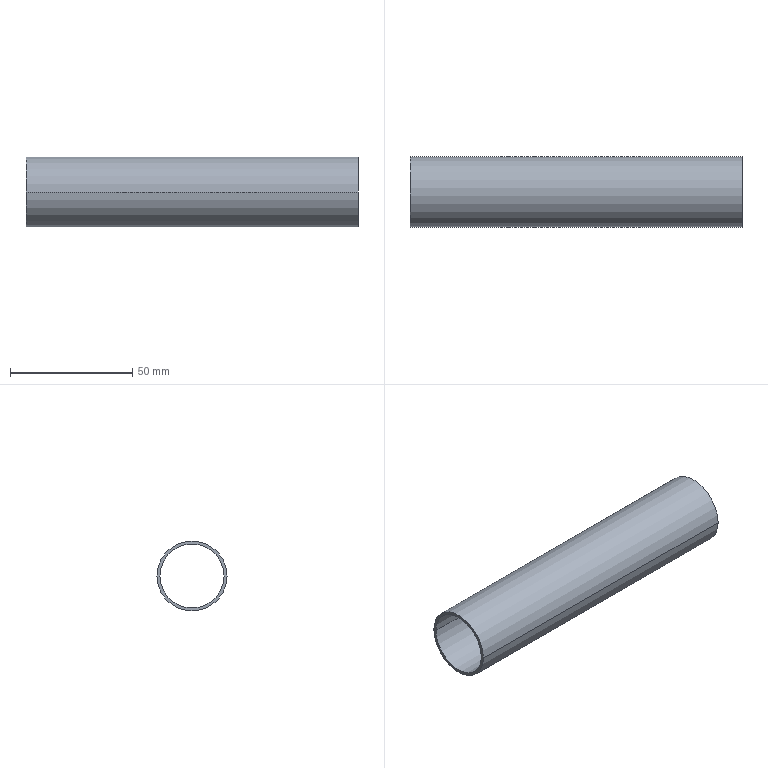Part | STEP file | TUBO REFUERZO CORTO_Predeterminado<Como mecanizada> | 1 solid | 6 faces | box 135.6 x 28.6 x 28.6 mm | volume 14007 mm3 | cylinder 4 | plane 2 | commonest cylinder face diameters 26.2 x2 28.6 x2
STEP:
#1=CARTESIAN_POINT('',(-67.8,-14.3,0.));
#2=VERTEX_POINT('',#1);
#3=CARTESIAN_POINT('',(-67.8,14.3,0.));
#4=VERTEX_POINT('',#3);
#5=CARTESIAN_POINT('',(-67.8,0.,0.));
#6=DIRECTION('',(-1.,0.,0.));
#7=DIRECTION('',(0.,-1.,0.));
#8=AXIS2_PLACEMENT_3D('',#5,#6,#7);
#9=CIRCLE('',#8,14.3);
#10=EDGE_CURVE('',#2,#4,#9,.T.);
#11=ORIENTED_EDGE('',*,*,#10,.F.);
#12=CARTESIAN_POINT('',(67.8,-14.3,0.));
#13=VERTEX_POINT('',#12);
#14=CARTESIAN_POINT('',(-67.8,-14.3,0.));
#15=DIRECTION('',(1.,0.,0.));
#16=VECTOR('',#15,1000.);
#17=LINE('',#14,#16);
#18=EDGE_CURVE('',#2,#13,#17,.T.);
#19=ORIENTED_EDGE('',*,*,#18,.T.);
#20=CARTESIAN_POINT('',(67.8,14.3,0.));
#21=VERTEX_POINT('',#20);
#22=CARTESIAN_POINT('',(67.8,0.,0.));
#23=DIRECTION('',(-1.,0.,0.));
#24=DIRECTION('',(0.,-1.,0.));
#25=AXIS2_PLACEMENT_3D('',#22,#23,#24);
#26=CIRCLE('',#25,14.3);
#27=EDGE_CURVE('',#13,#21,#26,.T.);
#28=ORIENTED_EDGE('',*,*,#27,.T.);
#29=CARTESIAN_POINT('',(-67.8,14.3,0.));
#30=DIRECTION('',(1.,0.,0.));
#31=VECTOR('',#30,1000.);
#32=LINE('',#29,#31);
#33=EDGE_CURVE('',#4,#21,#32,.T.);
#34=ORIENTED_EDGE('',*,*,#33,.F.);
#35=EDGE_LOOP('',(#11,#19,#28,#34));
#36=FACE_OUTER_BOUND('',#35,.T.);
#37=CARTESIAN_POINT('',(-67.8,0.,0.));
#38=DIRECTION('',(1.,0.,0.));
#39=DIRECTION('',(0.,1.,0.));
#40=AXIS2_PLACEMENT_3D('',#37,#38,#39);
#41=CYLINDRICAL_SURFACE('',#40,14.3);
#42=ADVANCED_FACE('',(#36),#41,.T.);
#43=CARTESIAN_POINT('',(-67.8,13.1,0.));
#44=VERTEX_POINT('',#43);
#45=CARTESIAN_POINT('',(-67.8,-13.1,0.));
#46=VERTEX_POINT('',#45);
#47=CARTESIAN_POINT('',(-67.8,0.,0.));
#48=DIRECTION('',(-1.,0.,0.));
#49=DIRECTION('',(0.,-1.,0.));
#50=AXIS2_PLACEMENT_3D('',#47,#48,#49);
#51=CIRCLE('',#50,13.1);
#52=EDGE_CURVE('',#44,#46,#51,.T.);
#53=ORIENTED_EDGE('',*,*,#52,.T.);
#54=CARTESIAN_POINT('',(67.8,-13.1,0.));
#55=VERTEX_POINT('',#54);
#56=CARTESIAN_POINT('',(-67.8,-13.1,0.));
#57=DIRECTION('',(1.,0.,0.));
#58=VECTOR('',#57,1000.);
#59=LINE('',#56,#58);
#60=EDGE_CURVE('',#46,#55,#59,.T.);
#61=ORIENTED_EDGE('',*,*,#60,.T.);
#62=CARTESIAN_POINT('',(67.8,13.1,0.));
#63=VERTEX_POINT('',#62);
#64=CARTESIAN_POINT('',(67.8,0.,0.));
#65=DIRECTION('',(-1.,0.,0.));
#66=DIRECTION('',(0.,-1.,0.));
#67=AXIS2_PLACEMENT_3D('',#64,#65,#66);
#68=CIRCLE('',#67,13.1);
#69=EDGE_CURVE('',#63,#55,#68,.T.);
#70=ORIENTED_EDGE('',*,*,#69,.F.);
#71=CARTESIAN_POINT('',(-67.8,13.1,0.));
#72=DIRECTION('',(1.,0.,0.));
#73=VECTOR('',#72,1000.);
#74=LINE('',#71,#73);
#75=EDGE_CURVE('',#44,#63,#74,.T.);
#76=ORIENTED_EDGE('',*,*,#75,.F.);
#77=EDGE_LOOP('',(#53,#61,#70,#76));
#78=FACE_OUTER_BOUND('',#77,.T.);
#79=CARTESIAN_POINT('',(-67.8,0.,0.));
#80=DIRECTION('',(1.,0.,0.));
#81=DIRECTION('',(0.,1.,0.));
#82=AXIS2_PLACEMENT_3D('',#79,#80,#81);
#83=CYLINDRICAL_SURFACE('',#82,13.1);
#84=ADVANCED_FACE('',(#78),#83,.F.);
#85=ORIENTED_EDGE('',*,*,#60,.F.);
#86=CARTESIAN_POINT('',(-67.8,0.,0.));
#87=DIRECTION('',(-1.,0.,0.));
#88=DIRECTION('',(0.,-1.,0.));
#89=AXIS2_PLACEMENT_3D('',#86,#87,#88);
#90=CIRCLE('',#89,13.1);
#91=EDGE_CURVE('',#46,#44,#90,.T.);
#92=ORIENTED_EDGE('',*,*,#91,.T.);
#93=ORIENTED_EDGE('',*,*,#75,.T.);
#94=CARTESIAN_POINT('',(67.8,0.,0.));
#95=DIRECTION('',(-1.,0.,0.));
#96=DIRECTION('',(0.,-1.,0.));
#97=AXIS2_PLACEMENT_3D('',#94,#95,#96);
#98=CIRCLE('',#97,13.1);
#99=EDGE_CURVE('',#55,#63,#98,.T.);
#100=ORIENTED_EDGE('',*,*,#99,.F.);
#101=EDGE_LOOP('',(#85,#92,#93,#100));
#102=FACE_OUTER_BOUND('',#101,.T.);
#103=CARTESIAN_POINT('',(-67.8,0.,0.));
#104=DIRECTION('',(1.,0.,0.));
#105=DIRECTION('',(0.,1.,0.));
#106=AXIS2_PLACEMENT_3D('',#103,#104,#105);
#107=CYLINDRICAL_SURFACE('',#106,13.1);
#108=ADVANCED_FACE('',(#102),#107,.F.);
#109=ORIENTED_EDGE('',*,*,#18,.F.);
#110=CARTESIAN_POINT('',(-67.8,0.,0.));
#111=DIRECTION('',(-1.,0.,0.));
#112=DIRECTION('',(0.,-1.,0.));
#113=AXIS2_PLACEMENT_3D('',#110,#111,#112);
#114=CIRCLE('',#113,14.3);
#115=EDGE_CURVE('',#4,#2,#114,.T.);
#116=ORIENTED_EDGE('',*,*,#115,.F.);
#117=ORIENTED_EDGE('',*,*,#33,.T.);
#118=CARTESIAN_POINT('',(67.8,0.,0.));
#119=DIRECTION('',(-1.,0.,0.));
#120=DIRECTION('',(0.,-1.,0.));
#121=AXIS2_PLACEMENT_3D('',#118,#119,#120);
#122=CIRCLE('',#121,14.3);
#123=EDGE_CURVE('',#21,#13,#122,.T.);
#124=ORIENTED_EDGE('',*,*,#123,.T.);
#125=EDGE_LOOP('',(#109,#116,#117,#124));
#126=FACE_OUTER_BOUND('',#125,.T.);
#127=CARTESIAN_POINT('',(-67.8,0.,0.));
#128=DIRECTION('',(1.,0.,0.));
#129=DIRECTION('',(0.,1.,0.));
#130=AXIS2_PLACEMENT_3D('',#127,#128,#129);
#131=CYLINDRICAL_SURFACE('',#130,14.3);
#132=ADVANCED_FACE('',(#126),#131,.T.);
#133=ORIENTED_EDGE('',*,*,#52,.F.);
#134=ORIENTED_EDGE('',*,*,#91,.F.);
#135=EDGE_LOOP('',(#133,#134));
#136=FACE_BOUND('',#135,.T.);
#137=ORIENTED_EDGE('',*,*,#115,.T.);
#138=ORIENTED_EDGE('',*,*,#10,.T.);
#139=EDGE_LOOP('',(#137,#138));
#140=FACE_OUTER_BOUND('',#139,.T.);
#141=CARTESIAN_POINT('',(-67.8,0.,0.));
#142=DIRECTION('',(-1.,0.,0.));
#143=DIRECTION('',(0.,-1.,0.));
#144=AXIS2_PLACEMENT_3D('',#141,#142,#143);
#145=PLANE('',#144);
#146=ADVANCED_FACE('',(#136,#140),#145,.T.);
#147=ORIENTED_EDGE('',*,*,#69,.T.);
#148=ORIENTED_EDGE('',*,*,#99,.T.);
#149=EDGE_LOOP('',(#147,#148));
#150=FACE_BOUND('',#149,.T.);
#151=ORIENTED_EDGE('',*,*,#123,.F.);
#152=ORIENTED_EDGE('',*,*,#27,.F.);
#153=EDGE_LOOP('',(#151,#152));
#154=FACE_OUTER_BOUND('',#153,.T.);
#155=CARTESIAN_POINT('',(67.8,0.,0.));
#156=DIRECTION('',(-1.,0.,0.));
#157=DIRECTION('',(0.,-1.,0.));
#158=AXIS2_PLACEMENT_3D('',#155,#156,#157);
#159=PLANE('',#158);
#160=ADVANCED_FACE('',(#150,#154),#159,.F.);
#161=CLOSED_SHELL('',(#42,#84,#108,#132,#146,#160));
#162=MANIFOLD_SOLID_BREP('',#161);
#163=CARTESIAN_POINT('',(0.,0.,0.));
#164=DIRECTION('',(0.,0.,1.));
#165=DIRECTION('',(1.,0.,0.));
#166=AXIS2_PLACEMENT_3D('',#163,#164,#165);
#167=(LENGTH_UNIT()NAMED_UNIT(*)SI_UNIT(.MILLI.,.METRE.));
#168=UNCERTAINTY_MEASURE_WITH_UNIT(LENGTH_MEASURE(0.00001),#167,'','');
#169=(NAMED_UNIT(*)PLANE_ANGLE_UNIT()SI_UNIT($,.RADIAN.));
#170=(NAMED_UNIT(*)SI_UNIT($,.STERADIAN.)SOLID_ANGLE_UNIT());
#171=(GEOMETRIC_REPRESENTATION_CONTEXT(3)GLOBAL_UNCERTAINTY_ASSIGNED_CONTEXT((#168))GLOBAL_UNIT_ASSIGNED_CONTEXT((#167,#169,#170))REPRESENTATION_CONTEXT('',''));
#172=ADVANCED_BREP_SHAPE_REPRESENTATION('',(#162,#166),#171);